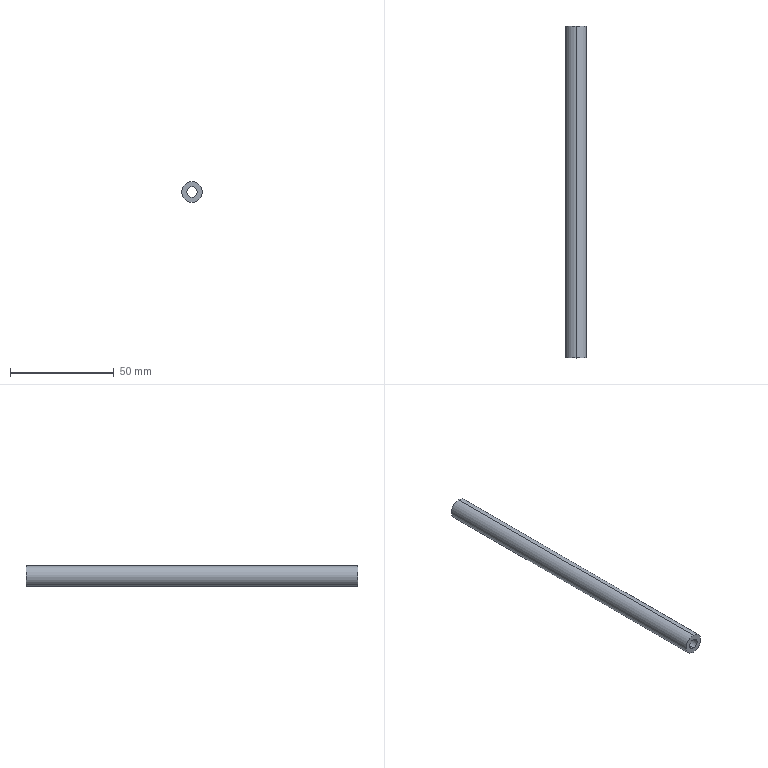Part | NX | features BREP 1 | 1 solid | 6 faces | box 10 x 160 x 10 mm | volume 9425 mm3 | cylinder 4 | plane 2 | commonest cylinder face diameters 5 x2 10 x2
STEP:
#1=CARTESIAN_POINT('',(0.,160.,-2.5));
#2=VERTEX_POINT('',#1);
#3=CARTESIAN_POINT('',(0.,160.,2.5));
#4=VERTEX_POINT('',#3);
#5=CARTESIAN_POINT('',(0.,160.,0.));
#6=DIRECTION('',(0.,1.,0.));
#7=DIRECTION('',(0.,0.,1.));
#8=AXIS2_PLACEMENT_3D('',#5,#6,#7);
#9=CIRCLE('',#8,2.5);
#10=EDGE_CURVE('',#2,#4,#9,.T.);
#11=ORIENTED_EDGE('',*,*,#10,.T.);
#12=CARTESIAN_POINT('',(0.,0.,2.5));
#13=VERTEX_POINT('',#12);
#14=CARTESIAN_POINT('',(0.,160.,2.5));
#15=DIRECTION('',(0.,-1.,0.));
#16=VECTOR('',#15,1000.);
#17=LINE('',#14,#16);
#18=EDGE_CURVE('',#13,#4,#17,.F.);
#19=ORIENTED_EDGE('',*,*,#18,.F.);
#20=CARTESIAN_POINT('',(0.,0.,-2.5));
#21=VERTEX_POINT('',#20);
#22=CARTESIAN_POINT('',(0.,0.,0.));
#23=DIRECTION('',(0.,1.,0.));
#24=DIRECTION('',(0.,0.,1.));
#25=AXIS2_PLACEMENT_3D('',#22,#23,#24);
#26=CIRCLE('',#25,2.5);
#27=EDGE_CURVE('',#21,#13,#26,.T.);
#28=ORIENTED_EDGE('',*,*,#27,.F.);
#29=CARTESIAN_POINT('',(0.,160.,-2.5));
#30=DIRECTION('',(0.,-1.,0.));
#31=VECTOR('',#30,1000.);
#32=LINE('',#29,#31);
#33=EDGE_CURVE('',#21,#2,#32,.F.);
#34=ORIENTED_EDGE('',*,*,#33,.T.);
#35=EDGE_LOOP('',(#11,#19,#28,#34));
#36=FACE_BOUND('',#35,.T.);
#37=CARTESIAN_POINT('',(0.,160.,0.));
#38=DIRECTION('',(0.,-1.,0.));
#39=DIRECTION('',(0.,0.,1.));
#40=AXIS2_PLACEMENT_3D('',#37,#38,#39);
#41=CYLINDRICAL_SURFACE('',#40,2.5);
#42=ADVANCED_FACE('',(#36),#41,.F.);
#43=CARTESIAN_POINT('',(0.,160.,5.));
#44=VERTEX_POINT('',#43);
#45=CARTESIAN_POINT('',(0.,160.,-5.));
#46=VERTEX_POINT('',#45);
#47=CARTESIAN_POINT('',(0.,160.,0.));
#48=DIRECTION('',(0.,1.,0.));
#49=DIRECTION('',(0.,0.,1.));
#50=AXIS2_PLACEMENT_3D('',#47,#48,#49);
#51=CIRCLE('',#50,5.);
#52=EDGE_CURVE('',#44,#46,#51,.T.);
#53=ORIENTED_EDGE('',*,*,#52,.F.);
#54=CARTESIAN_POINT('',(0.,0.,5.));
#55=VERTEX_POINT('',#54);
#56=CARTESIAN_POINT('',(0.,160.,5.));
#57=DIRECTION('',(0.,-1.,0.));
#58=VECTOR('',#57,1000.);
#59=LINE('',#56,#58);
#60=EDGE_CURVE('',#55,#44,#59,.F.);
#61=ORIENTED_EDGE('',*,*,#60,.F.);
#62=CARTESIAN_POINT('',(0.,0.,-5.));
#63=VERTEX_POINT('',#62);
#64=CARTESIAN_POINT('',(0.,0.,0.));
#65=DIRECTION('',(0.,1.,0.));
#66=DIRECTION('',(0.,0.,1.));
#67=AXIS2_PLACEMENT_3D('',#64,#65,#66);
#68=CIRCLE('',#67,5.);
#69=EDGE_CURVE('',#55,#63,#68,.T.);
#70=ORIENTED_EDGE('',*,*,#69,.T.);
#71=CARTESIAN_POINT('',(0.,160.,-5.));
#72=DIRECTION('',(0.,-1.,0.));
#73=VECTOR('',#72,1000.);
#74=LINE('',#71,#73);
#75=EDGE_CURVE('',#63,#46,#74,.F.);
#76=ORIENTED_EDGE('',*,*,#75,.T.);
#77=EDGE_LOOP('',(#53,#61,#70,#76));
#78=FACE_BOUND('',#77,.T.);
#79=CARTESIAN_POINT('',(0.,160.,0.));
#80=DIRECTION('',(0.,-1.,0.));
#81=DIRECTION('',(0.,0.,1.));
#82=AXIS2_PLACEMENT_3D('',#79,#80,#81);
#83=CYLINDRICAL_SURFACE('',#82,5.);
#84=ADVANCED_FACE('',(#78),#83,.T.);
#85=CARTESIAN_POINT('',(0.,160.,0.));
#86=DIRECTION('',(0.,1.,0.));
#87=DIRECTION('',(0.,0.,1.));
#88=AXIS2_PLACEMENT_3D('',#85,#86,#87);
#89=CIRCLE('',#88,5.);
#90=EDGE_CURVE('',#46,#44,#89,.T.);
#91=ORIENTED_EDGE('',*,*,#90,.T.);
#92=ORIENTED_EDGE('',*,*,#52,.T.);
#93=EDGE_LOOP('',(#91,#92));
#94=FACE_BOUND('',#93,.T.);
#95=ORIENTED_EDGE('',*,*,#10,.F.);
#96=CARTESIAN_POINT('',(0.,160.,0.));
#97=DIRECTION('',(0.,1.,0.));
#98=DIRECTION('',(0.,0.,1.));
#99=AXIS2_PLACEMENT_3D('',#96,#97,#98);
#100=CIRCLE('',#99,2.5);
#101=EDGE_CURVE('',#4,#2,#100,.T.);
#102=ORIENTED_EDGE('',*,*,#101,.F.);
#103=EDGE_LOOP('',(#95,#102));
#104=FACE_BOUND('',#103,.T.);
#105=CARTESIAN_POINT('',(0.,160.,0.));
#106=DIRECTION('',(0.,1.,0.));
#107=DIRECTION('',(0.,0.,1.));
#108=AXIS2_PLACEMENT_3D('',#105,#106,#107);
#109=PLANE('',#108);
#110=ADVANCED_FACE('',(#94,#104),#109,.T.);
#111=CARTESIAN_POINT('',(0.,0.,0.));
#112=DIRECTION('',(0.,1.,0.));
#113=DIRECTION('',(0.,0.,1.));
#114=AXIS2_PLACEMENT_3D('',#111,#112,#113);
#115=CIRCLE('',#114,5.);
#116=EDGE_CURVE('',#63,#55,#115,.T.);
#117=ORIENTED_EDGE('',*,*,#116,.F.);
#118=ORIENTED_EDGE('',*,*,#69,.F.);
#119=EDGE_LOOP('',(#117,#118));
#120=FACE_BOUND('',#119,.T.);
#121=ORIENTED_EDGE('',*,*,#27,.T.);
#122=CARTESIAN_POINT('',(0.,0.,0.));
#123=DIRECTION('',(0.,1.,0.));
#124=DIRECTION('',(0.,0.,1.));
#125=AXIS2_PLACEMENT_3D('',#122,#123,#124);
#126=CIRCLE('',#125,2.5);
#127=EDGE_CURVE('',#13,#21,#126,.T.);
#128=ORIENTED_EDGE('',*,*,#127,.T.);
#129=EDGE_LOOP('',(#121,#128));
#130=FACE_BOUND('',#129,.T.);
#131=CARTESIAN_POINT('',(0.,0.,0.));
#132=DIRECTION('',(0.,1.,0.));
#133=DIRECTION('',(0.,0.,1.));
#134=AXIS2_PLACEMENT_3D('',#131,#132,#133);
#135=PLANE('',#134);
#136=ADVANCED_FACE('',(#120,#130),#135,.F.);
#137=ORIENTED_EDGE('',*,*,#60,.T.);
#138=ORIENTED_EDGE('',*,*,#90,.F.);
#139=ORIENTED_EDGE('',*,*,#75,.F.);
#140=ORIENTED_EDGE('',*,*,#116,.T.);
#141=EDGE_LOOP('',(#137,#138,#139,#140));
#142=FACE_BOUND('',#141,.T.);
#143=CARTESIAN_POINT('',(0.,160.,0.));
#144=DIRECTION('',(0.,-1.,0.));
#145=DIRECTION('',(0.,0.,1.));
#146=AXIS2_PLACEMENT_3D('',#143,#144,#145);
#147=CYLINDRICAL_SURFACE('',#146,5.);
#148=ADVANCED_FACE('',(#142),#147,.T.);
#149=ORIENTED_EDGE('',*,*,#18,.T.);
#150=ORIENTED_EDGE('',*,*,#101,.T.);
#151=ORIENTED_EDGE('',*,*,#33,.F.);
#152=ORIENTED_EDGE('',*,*,#127,.F.);
#153=EDGE_LOOP('',(#149,#150,#151,#152));
#154=FACE_BOUND('',#153,.T.);
#155=CARTESIAN_POINT('',(0.,160.,0.));
#156=DIRECTION('',(0.,-1.,0.));
#157=DIRECTION('',(0.,0.,1.));
#158=AXIS2_PLACEMENT_3D('',#155,#156,#157);
#159=CYLINDRICAL_SURFACE('',#158,2.5);
#160=ADVANCED_FACE('',(#154),#159,.F.);
#161=CLOSED_SHELL('',(#42,#84,#110,#136,#148,#160));
#162=MANIFOLD_SOLID_BREP('',#161);
#163=(LENGTH_UNIT()NAMED_UNIT(*)SI_UNIT(.MILLI.,.METRE.));
#164=UNCERTAINTY_MEASURE_WITH_UNIT(LENGTH_MEASURE(0.00001),#163,'','');
#165=(NAMED_UNIT(*)PLANE_ANGLE_UNIT()SI_UNIT($,.RADIAN.));
#166=(NAMED_UNIT(*)SI_UNIT($,.STERADIAN.)SOLID_ANGLE_UNIT());
#167=(GEOMETRIC_REPRESENTATION_CONTEXT(3)GLOBAL_UNCERTAINTY_ASSIGNED_CONTEXT((#164))GLOBAL_UNIT_ASSIGNED_CONTEXT((#163,#165,#166))REPRESENTATION_CONTEXT('',''));
#168=ADVANCED_BREP_SHAPE_REPRESENTATION('',(#162),#167);